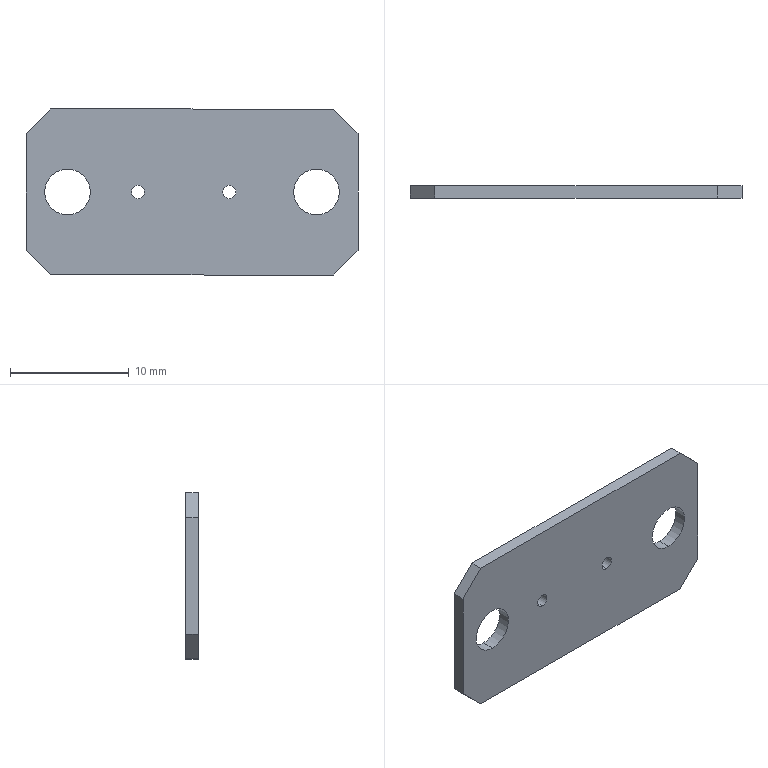Part | SolidWorks | features SplitBody 1 | 1 solid | 18 faces | box 28 x 1.05 x 14 mm | volume 375.823 mm3 | plane 10 | cylinder 8 | commonest cylinder face diameters 1.12 x4 3.85 x4
STEP:
#1=CARTESIAN_POINT('',(336.575,257.909,-266.241));
#2=VERTEX_POINT('',#1);
#3=CARTESIAN_POINT('',(336.575,257.909,-262.391));
#4=VERTEX_POINT('',#3);
#5=CARTESIAN_POINT('',(336.575,257.909,-264.316));
#6=DIRECTION('',(0.,-1.,0.));
#7=DIRECTION('',(0.,0.,1.));
#8=AXIS2_PLACEMENT_3D('',#5,#6,#7);
#9=CIRCLE('',#8,1.925);
#10=EDGE_CURVE('',#2,#4,#9,.T.);
#11=ORIENTED_EDGE('',*,*,#10,.F.);
#12=CARTESIAN_POINT('',(336.575,256.859,-266.241));
#13=VERTEX_POINT('',#12);
#14=CARTESIAN_POINT('',(336.575,263.859,-266.241));
#15=DIRECTION('',(0.,-1.,0.));
#16=VECTOR('',#15,1000.);
#17=LINE('',#14,#16);
#18=EDGE_CURVE('',#2,#13,#17,.T.);
#19=ORIENTED_EDGE('',*,*,#18,.T.);
#20=CARTESIAN_POINT('',(336.575,256.859,-262.391));
#21=VERTEX_POINT('',#20);
#22=CARTESIAN_POINT('',(336.575,256.859,-264.316));
#23=DIRECTION('',(0.,-1.,0.));
#24=DIRECTION('',(0.,0.,1.));
#25=AXIS2_PLACEMENT_3D('',#22,#23,#24);
#26=CIRCLE('',#25,1.925);
#27=EDGE_CURVE('',#13,#21,#26,.T.);
#28=ORIENTED_EDGE('',*,*,#27,.T.);
#29=CARTESIAN_POINT('',(336.575,263.859,-262.391));
#30=DIRECTION('',(0.,-1.,0.));
#31=VECTOR('',#30,1000.);
#32=LINE('',#29,#31);
#33=EDGE_CURVE('',#4,#21,#32,.T.);
#34=ORIENTED_EDGE('',*,*,#33,.F.);
#35=EDGE_LOOP('',(#11,#19,#28,#34));
#36=FACE_OUTER_BOUND('',#35,.T.);
#37=CARTESIAN_POINT('',(336.575,263.859,-264.316));
#38=DIRECTION('',(0.,-1.,0.));
#39=DIRECTION('',(0.,0.,1.));
#40=AXIS2_PLACEMENT_3D('',#37,#38,#39);
#41=CYLINDRICAL_SURFACE('',#40,1.925);
#42=ADVANCED_FACE('',(#36),#41,.F.);
#43=CARTESIAN_POINT('',(315.575,257.909,-266.241));
#44=VERTEX_POINT('',#43);
#45=CARTESIAN_POINT('',(315.575,257.909,-262.391));
#46=VERTEX_POINT('',#45);
#47=CARTESIAN_POINT('',(315.575,257.909,-264.316));
#48=DIRECTION('',(0.,-1.,0.));
#49=DIRECTION('',(0.,0.,1.));
#50=AXIS2_PLACEMENT_3D('',#47,#48,#49);
#51=CIRCLE('',#50,1.925);
#52=EDGE_CURVE('',#44,#46,#51,.T.);
#53=ORIENTED_EDGE('',*,*,#52,.F.);
#54=CARTESIAN_POINT('',(315.575,256.859,-266.241));
#55=VERTEX_POINT('',#54);
#56=CARTESIAN_POINT('',(315.575,263.859,-266.241));
#57=DIRECTION('',(0.,-1.,0.));
#58=VECTOR('',#57,1000.);
#59=LINE('',#56,#58);
#60=EDGE_CURVE('',#44,#55,#59,.T.);
#61=ORIENTED_EDGE('',*,*,#60,.T.);
#62=CARTESIAN_POINT('',(315.575,256.859,-262.391));
#63=VERTEX_POINT('',#62);
#64=CARTESIAN_POINT('',(315.575,256.859,-264.316));
#65=DIRECTION('',(0.,-1.,0.));
#66=DIRECTION('',(0.,0.,1.));
#67=AXIS2_PLACEMENT_3D('',#64,#65,#66);
#68=CIRCLE('',#67,1.925);
#69=EDGE_CURVE('',#55,#63,#68,.T.);
#70=ORIENTED_EDGE('',*,*,#69,.T.);
#71=CARTESIAN_POINT('',(315.575,263.859,-262.391));
#72=DIRECTION('',(0.,-1.,0.));
#73=VECTOR('',#72,1000.);
#74=LINE('',#71,#73);
#75=EDGE_CURVE('',#46,#63,#74,.T.);
#76=ORIENTED_EDGE('',*,*,#75,.F.);
#77=EDGE_LOOP('',(#53,#61,#70,#76));
#78=FACE_OUTER_BOUND('',#77,.T.);
#79=CARTESIAN_POINT('',(315.575,263.859,-264.316));
#80=DIRECTION('',(0.,-1.,0.));
#81=DIRECTION('',(0.,0.,1.));
#82=AXIS2_PLACEMENT_3D('',#79,#80,#81);
#83=CYLINDRICAL_SURFACE('',#82,1.925);
#84=ADVANCED_FACE('',(#78),#83,.F.);
#85=CARTESIAN_POINT('',(321.525,257.909,-264.876));
#86=VERTEX_POINT('',#85);
#87=CARTESIAN_POINT('',(321.525,257.909,-263.756));
#88=VERTEX_POINT('',#87);
#89=CARTESIAN_POINT('',(321.525,257.909,-264.316));
#90=DIRECTION('',(0.,-1.,0.));
#91=DIRECTION('',(0.,0.,1.));
#92=AXIS2_PLACEMENT_3D('',#89,#90,#91);
#93=CIRCLE('',#92,0.56);
#94=EDGE_CURVE('',#86,#88,#93,.T.);
#95=ORIENTED_EDGE('',*,*,#94,.F.);
#96=CARTESIAN_POINT('',(321.525,256.859,-264.876));
#97=VERTEX_POINT('',#96);
#98=CARTESIAN_POINT('',(321.525,256.859,-264.876));
#99=DIRECTION('',(0.,-1.,0.));
#100=VECTOR('',#99,1000.);
#101=LINE('',#98,#100);
#102=EDGE_CURVE('',#86,#97,#101,.T.);
#103=ORIENTED_EDGE('',*,*,#102,.T.);
#104=CARTESIAN_POINT('',(321.525,256.859,-263.756));
#105=VERTEX_POINT('',#104);
#106=CARTESIAN_POINT('',(321.525,256.859,-264.316));
#107=DIRECTION('',(0.,-1.,0.));
#108=DIRECTION('',(0.,0.,1.));
#109=AXIS2_PLACEMENT_3D('',#106,#107,#108);
#110=CIRCLE('',#109,0.56);
#111=EDGE_CURVE('',#97,#105,#110,.T.);
#112=ORIENTED_EDGE('',*,*,#111,.T.);
#113=CARTESIAN_POINT('',(321.525,256.859,-263.756));
#114=DIRECTION('',(0.,-1.,0.));
#115=VECTOR('',#114,1000.);
#116=LINE('',#113,#115);
#117=EDGE_CURVE('',#88,#105,#116,.T.);
#118=ORIENTED_EDGE('',*,*,#117,.F.);
#119=EDGE_LOOP('',(#95,#103,#112,#118));
#120=FACE_OUTER_BOUND('',#119,.T.);
#121=CARTESIAN_POINT('',(321.525,256.859,-264.316));
#122=DIRECTION('',(0.,-1.,0.));
#123=DIRECTION('',(0.,0.,1.));
#124=AXIS2_PLACEMENT_3D('',#121,#122,#123);
#125=CYLINDRICAL_SURFACE('',#124,0.56);
#126=ADVANCED_FACE('',(#120),#125,.F.);
#127=CARTESIAN_POINT('',(329.225,257.909,-264.876));
#128=VERTEX_POINT('',#127);
#129=CARTESIAN_POINT('',(329.225,257.909,-263.756));
#130=VERTEX_POINT('',#129);
#131=CARTESIAN_POINT('',(329.225,257.909,-264.316));
#132=DIRECTION('',(0.,-1.,0.));
#133=DIRECTION('',(0.,0.,1.));
#134=AXIS2_PLACEMENT_3D('',#131,#132,#133);
#135=CIRCLE('',#134,0.56);
#136=EDGE_CURVE('',#128,#130,#135,.T.);
#137=ORIENTED_EDGE('',*,*,#136,.F.);
#138=CARTESIAN_POINT('',(329.225,256.859,-264.876));
#139=VERTEX_POINT('',#138);
#140=CARTESIAN_POINT('',(329.225,256.859,-264.876));
#141=DIRECTION('',(0.,-1.,0.));
#142=VECTOR('',#141,1000.);
#143=LINE('',#140,#142);
#144=EDGE_CURVE('',#128,#139,#143,.T.);
#145=ORIENTED_EDGE('',*,*,#144,.T.);
#146=CARTESIAN_POINT('',(329.225,256.859,-263.756));
#147=VERTEX_POINT('',#146);
#148=CARTESIAN_POINT('',(329.225,256.859,-264.316));
#149=DIRECTION('',(0.,-1.,0.));
#150=DIRECTION('',(0.,0.,1.));
#151=AXIS2_PLACEMENT_3D('',#148,#149,#150);
#152=CIRCLE('',#151,0.56);
#153=EDGE_CURVE('',#139,#147,#152,.T.);
#154=ORIENTED_EDGE('',*,*,#153,.T.);
#155=CARTESIAN_POINT('',(329.225,256.859,-263.756));
#156=DIRECTION('',(0.,-1.,0.));
#157=VECTOR('',#156,1000.);
#158=LINE('',#155,#157);
#159=EDGE_CURVE('',#130,#147,#158,.T.);
#160=ORIENTED_EDGE('',*,*,#159,.F.);
#161=EDGE_LOOP('',(#137,#145,#154,#160));
#162=FACE_OUTER_BOUND('',#161,.T.);
#163=CARTESIAN_POINT('',(329.225,256.859,-264.316));
#164=DIRECTION('',(0.,-1.,0.));
#165=DIRECTION('',(0.,0.,1.));
#166=AXIS2_PLACEMENT_3D('',#163,#164,#165);
#167=CYLINDRICAL_SURFACE('',#166,0.56);
#168=ADVANCED_FACE('',(#162),#167,.F.);
#169=CARTESIAN_POINT('',(314.175,256.859,-271.316));
#170=VERTEX_POINT('',#169);
#171=CARTESIAN_POINT('',(337.975,256.859,-271.316));
#172=VERTEX_POINT('',#171);
#173=CARTESIAN_POINT('',(312.075,256.859,-271.316));
#174=DIRECTION('',(1.,0.,0.));
#175=VECTOR('',#174,1000.);
#176=LINE('',#173,#175);
#177=EDGE_CURVE('',#170,#172,#176,.T.);
#178=ORIENTED_EDGE('',*,*,#177,.F.);
#179=CARTESIAN_POINT('',(314.175,257.909,-271.316));
#180=VERTEX_POINT('',#179);
#181=CARTESIAN_POINT('',(314.175,256.859,-271.316));
#182=DIRECTION('',(0.,1.,0.));
#183=VECTOR('',#182,1000.);
#184=LINE('',#181,#183);
#185=EDGE_CURVE('',#170,#180,#184,.T.);
#186=ORIENTED_EDGE('',*,*,#185,.T.);
#187=CARTESIAN_POINT('',(337.975,257.909,-271.316));
#188=VERTEX_POINT('',#187);
#189=CARTESIAN_POINT('',(312.075,257.909,-271.316));
#190=DIRECTION('',(1.,0.,0.));
#191=VECTOR('',#190,1000.);
#192=LINE('',#189,#191);
#193=EDGE_CURVE('',#180,#188,#192,.T.);
#194=ORIENTED_EDGE('',*,*,#193,.T.);
#195=CARTESIAN_POINT('',(337.975,256.859,-271.316));
#196=DIRECTION('',(0.,-1.,0.));
#197=VECTOR('',#196,1000.);
#198=LINE('',#195,#197);
#199=EDGE_CURVE('',#188,#172,#198,.T.);
#200=ORIENTED_EDGE('',*,*,#199,.T.);
#201=EDGE_LOOP('',(#178,#186,#194,#200));
#202=FACE_OUTER_BOUND('',#201,.T.);
#203=CARTESIAN_POINT('',(312.075,256.859,-271.316));
#204=DIRECTION('',(0.,0.,1.));
#205=DIRECTION('',(-1.,0.,0.));
#206=AXIS2_PLACEMENT_3D('',#203,#204,#205);
#207=PLANE('',#206);
#208=ADVANCED_FACE('',(#202),#207,.F.);
#209=CARTESIAN_POINT('',(340.075,257.909,-269.216));
#210=VERTEX_POINT('',#209);
#211=CARTESIAN_POINT('',(340.075,257.909,-259.416));
#212=VERTEX_POINT('',#211);
#213=CARTESIAN_POINT('',(340.075,257.909,-271.316));
#214=DIRECTION('',(0.,0.,1.));
#215=VECTOR('',#214,1000.);
#216=LINE('',#213,#215);
#217=EDGE_CURVE('',#210,#212,#216,.T.);
#218=ORIENTED_EDGE('',*,*,#217,.T.);
#219=CARTESIAN_POINT('',(340.075,256.859,-259.416));
#220=VERTEX_POINT('',#219);
#221=CARTESIAN_POINT('',(340.075,256.859,-259.416));
#222=DIRECTION('',(0.,-1.,0.));
#223=VECTOR('',#222,1000.);
#224=LINE('',#221,#223);
#225=EDGE_CURVE('',#212,#220,#224,.T.);
#226=ORIENTED_EDGE('',*,*,#225,.T.);
#227=CARTESIAN_POINT('',(340.075,256.859,-269.216));
#228=VERTEX_POINT('',#227);
#229=CARTESIAN_POINT('',(340.075,256.859,-271.316));
#230=DIRECTION('',(0.,0.,1.));
#231=VECTOR('',#230,1000.);
#232=LINE('',#229,#231);
#233=EDGE_CURVE('',#228,#220,#232,.T.);
#234=ORIENTED_EDGE('',*,*,#233,.F.);
#235=CARTESIAN_POINT('',(340.075,256.859,-269.216));
#236=DIRECTION('',(0.,1.,0.));
#237=VECTOR('',#236,1000.);
#238=LINE('',#235,#237);
#239=EDGE_CURVE('',#228,#210,#238,.T.);
#240=ORIENTED_EDGE('',*,*,#239,.T.);
#241=EDGE_LOOP('',(#218,#226,#234,#240));
#242=FACE_OUTER_BOUND('',#241,.T.);
#243=CARTESIAN_POINT('',(340.075,256.859,-271.316));
#244=DIRECTION('',(-1.,0.,0.));
#245=DIRECTION('',(0.,-1.,0.));
#246=AXIS2_PLACEMENT_3D('',#243,#244,#245);
#247=PLANE('',#246);
#248=ADVANCED_FACE('',(#242),#247,.F.);
#249=CARTESIAN_POINT('',(337.975,257.909,-257.316));
#250=VERTEX_POINT('',#249);
#251=CARTESIAN_POINT('',(314.175,257.909,-257.316));
#252=VERTEX_POINT('',#251);
#253=CARTESIAN_POINT('',(312.075,257.909,-257.316));
#254=DIRECTION('',(-1.,0.,0.));
#255=VECTOR('',#254,1000.);
#256=LINE('',#253,#255);
#257=EDGE_CURVE('',#250,#252,#256,.T.);
#258=ORIENTED_EDGE('',*,*,#257,.T.);
#259=CARTESIAN_POINT('',(314.175,256.859,-257.316));
#260=VERTEX_POINT('',#259);
#261=CARTESIAN_POINT('',(314.175,256.859,-257.316));
#262=DIRECTION('',(0.,-1.,0.));
#263=VECTOR('',#262,1000.);
#264=LINE('',#261,#263);
#265=EDGE_CURVE('',#252,#260,#264,.T.);
#266=ORIENTED_EDGE('',*,*,#265,.T.);
#267=CARTESIAN_POINT('',(337.975,256.859,-257.316));
#268=VERTEX_POINT('',#267);
#269=CARTESIAN_POINT('',(312.075,256.859,-257.316));
#270=DIRECTION('',(-1.,0.,0.));
#271=VECTOR('',#270,1000.);
#272=LINE('',#269,#271);
#273=EDGE_CURVE('',#268,#260,#272,.T.);
#274=ORIENTED_EDGE('',*,*,#273,.F.);
#275=CARTESIAN_POINT('',(337.975,256.859,-257.316));
#276=DIRECTION('',(0.,1.,0.));
#277=VECTOR('',#276,1000.);
#278=LINE('',#275,#277);
#279=EDGE_CURVE('',#268,#250,#278,.T.);
#280=ORIENTED_EDGE('',*,*,#279,.T.);
#281=EDGE_LOOP('',(#258,#266,#274,#280));
#282=FACE_OUTER_BOUND('',#281,.T.);
#283=CARTESIAN_POINT('',(312.075,256.859,-257.316));
#284=DIRECTION('',(0.,0.,-1.));
#285=DIRECTION('',(1.,0.,0.));
#286=AXIS2_PLACEMENT_3D('',#283,#284,#285);
#287=PLANE('',#286);
#288=ADVANCED_FACE('',(#282),#287,.F.);
#289=CARTESIAN_POINT('',(312.075,257.909,-259.416));
#290=VERTEX_POINT('',#289);
#291=CARTESIAN_POINT('',(312.075,257.909,-269.216));
#292=VERTEX_POINT('',#291);
#293=CARTESIAN_POINT('',(312.075,257.909,-271.316));
#294=DIRECTION('',(0.,0.,-1.));
#295=VECTOR('',#294,1000.);
#296=LINE('',#293,#295);
#297=EDGE_CURVE('',#290,#292,#296,.T.);
#298=ORIENTED_EDGE('',*,*,#297,.T.);
#299=CARTESIAN_POINT('',(312.075,256.859,-269.216));
#300=VERTEX_POINT('',#299);
#301=CARTESIAN_POINT('',(312.075,256.859,-269.216));
#302=DIRECTION('',(0.,-1.,0.));
#303=VECTOR('',#302,1000.);
#304=LINE('',#301,#303);
#305=EDGE_CURVE('',#292,#300,#304,.T.);
#306=ORIENTED_EDGE('',*,*,#305,.T.);
#307=CARTESIAN_POINT('',(312.075,256.859,-259.416));
#308=VERTEX_POINT('',#307);
#309=CARTESIAN_POINT('',(312.075,256.859,-271.316));
#310=DIRECTION('',(0.,0.,-1.));
#311=VECTOR('',#310,1000.);
#312=LINE('',#309,#311);
#313=EDGE_CURVE('',#308,#300,#312,.T.);
#314=ORIENTED_EDGE('',*,*,#313,.F.);
#315=CARTESIAN_POINT('',(312.075,256.859,-259.416));
#316=DIRECTION('',(0.,1.,0.));
#317=VECTOR('',#316,1000.);
#318=LINE('',#315,#317);
#319=EDGE_CURVE('',#308,#290,#318,.T.);
#320=ORIENTED_EDGE('',*,*,#319,.T.);
#321=EDGE_LOOP('',(#298,#306,#314,#320));
#322=FACE_OUTER_BOUND('',#321,.T.);
#323=CARTESIAN_POINT('',(312.075,256.859,-271.316));
#324=DIRECTION('',(1.,0.,0.));
#325=DIRECTION('',(0.,1.,0.));
#326=AXIS2_PLACEMENT_3D('',#323,#324,#325);
#327=PLANE('',#326);
#328=ADVANCED_FACE('',(#322),#327,.F.);
#329=CARTESIAN_POINT('',(336.575,256.859,-264.316));
#330=DIRECTION('',(0.,-1.,0.));
#331=DIRECTION('',(0.,0.,1.));
#332=AXIS2_PLACEMENT_3D('',#329,#330,#331);
#333=CIRCLE('',#332,1.925);
#334=EDGE_CURVE('',#21,#13,#333,.T.);
#335=ORIENTED_EDGE('',*,*,#334,.F.);
#336=ORIENTED_EDGE('',*,*,#27,.F.);
#337=EDGE_LOOP('',(#335,#336));
#338=FACE_BOUND('',#337,.T.);
#339=CARTESIAN_POINT('',(315.575,256.859,-264.316));
#340=DIRECTION('',(0.,-1.,0.));
#341=DIRECTION('',(0.,0.,1.));
#342=AXIS2_PLACEMENT_3D('',#339,#340,#341);
#343=CIRCLE('',#342,1.925);
#344=EDGE_CURVE('',#63,#55,#343,.T.);
#345=ORIENTED_EDGE('',*,*,#344,.F.);
#346=ORIENTED_EDGE('',*,*,#69,.F.);
#347=EDGE_LOOP('',(#345,#346));
#348=FACE_BOUND('',#347,.T.);
#349=CARTESIAN_POINT('',(321.525,256.859,-264.316));
#350=DIRECTION('',(0.,-1.,0.));
#351=DIRECTION('',(0.,0.,1.));
#352=AXIS2_PLACEMENT_3D('',#349,#350,#351);
#353=CIRCLE('',#352,0.56);
#354=EDGE_CURVE('',#105,#97,#353,.T.);
#355=ORIENTED_EDGE('',*,*,#354,.F.);
#356=ORIENTED_EDGE('',*,*,#111,.F.);
#357=EDGE_LOOP('',(#355,#356));
#358=FACE_BOUND('',#357,.T.);
#359=CARTESIAN_POINT('',(329.225,256.859,-264.316));
#360=DIRECTION('',(0.,-1.,0.));
#361=DIRECTION('',(0.,0.,1.));
#362=AXIS2_PLACEMENT_3D('',#359,#360,#361);
#363=CIRCLE('',#362,0.56);
#364=EDGE_CURVE('',#147,#139,#363,.T.);
#365=ORIENTED_EDGE('',*,*,#364,.F.);
#366=ORIENTED_EDGE('',*,*,#153,.F.);
#367=EDGE_LOOP('',(#365,#366));
#368=FACE_BOUND('',#367,.T.);
#369=ORIENTED_EDGE('',*,*,#313,.T.);
#370=CARTESIAN_POINT('',(327.125,256.859,-284.266));
#371=DIRECTION('',(0.7071,0.,-0.7071));
#372=VECTOR('',#371,1000.);
#373=LINE('',#370,#372);
#374=EDGE_CURVE('',#300,#170,#373,.T.);
#375=ORIENTED_EDGE('',*,*,#374,.T.);
#376=ORIENTED_EDGE('',*,*,#177,.T.);
#377=CARTESIAN_POINT('',(339.025,256.859,-270.266));
#378=DIRECTION('',(0.7071,0.,0.7071));
#379=VECTOR('',#378,1000.);
#380=LINE('',#377,#379);
#381=EDGE_CURVE('',#172,#228,#380,.T.);
#382=ORIENTED_EDGE('',*,*,#381,.T.);
#383=ORIENTED_EDGE('',*,*,#233,.T.);
#384=CARTESIAN_POINT('',(346.025,256.859,-265.366));
#385=DIRECTION('',(-0.7071,0.,0.7071));
#386=VECTOR('',#385,1000.);
#387=LINE('',#384,#386);
#388=EDGE_CURVE('',#220,#268,#387,.T.);
#389=ORIENTED_EDGE('',*,*,#388,.T.);
#390=ORIENTED_EDGE('',*,*,#273,.T.);
#391=CARTESIAN_POINT('',(320.125,256.859,-251.366));
#392=DIRECTION('',(-0.7071,0.,-0.7071));
#393=VECTOR('',#392,1000.);
#394=LINE('',#391,#393);
#395=EDGE_CURVE('',#260,#308,#394,.T.);
#396=ORIENTED_EDGE('',*,*,#395,.T.);
#397=EDGE_LOOP('',(#369,#375,#376,#382,#383,#389,#390,#396));
#398=FACE_OUTER_BOUND('',#397,.T.);
#399=CARTESIAN_POINT('',(340.075,256.859,-271.316));
#400=DIRECTION('',(0.,-1.,0.));
#401=DIRECTION('',(0.,0.,1.));
#402=AXIS2_PLACEMENT_3D('',#399,#400,#401);
#403=PLANE('',#402);
#404=ADVANCED_FACE('',(#338,#348,#358,#368,#398),#403,.T.);
#405=CARTESIAN_POINT('',(336.575,257.909,-264.316));
#406=DIRECTION('',(0.,-1.,0.));
#407=DIRECTION('',(0.,0.,1.));
#408=AXIS2_PLACEMENT_3D('',#405,#406,#407);
#409=CIRCLE('',#408,1.925);
#410=EDGE_CURVE('',#4,#2,#409,.T.);
#411=ORIENTED_EDGE('',*,*,#410,.T.);
#412=ORIENTED_EDGE('',*,*,#10,.T.);
#413=EDGE_LOOP('',(#411,#412));
#414=FACE_BOUND('',#413,.T.);
#415=CARTESIAN_POINT('',(315.575,257.909,-264.316));
#416=DIRECTION('',(0.,-1.,0.));
#417=DIRECTION('',(0.,0.,1.));
#418=AXIS2_PLACEMENT_3D('',#415,#416,#417);
#419=CIRCLE('',#418,1.925);
#420=EDGE_CURVE('',#46,#44,#419,.T.);
#421=ORIENTED_EDGE('',*,*,#420,.T.);
#422=ORIENTED_EDGE('',*,*,#52,.T.);
#423=EDGE_LOOP('',(#421,#422));
#424=FACE_BOUND('',#423,.T.);
#425=CARTESIAN_POINT('',(321.525,257.909,-264.316));
#426=DIRECTION('',(0.,-1.,0.));
#427=DIRECTION('',(0.,0.,1.));
#428=AXIS2_PLACEMENT_3D('',#425,#426,#427);
#429=CIRCLE('',#428,0.56);
#430=EDGE_CURVE('',#88,#86,#429,.T.);
#431=ORIENTED_EDGE('',*,*,#430,.T.);
#432=ORIENTED_EDGE('',*,*,#94,.T.);
#433=EDGE_LOOP('',(#431,#432));
#434=FACE_BOUND('',#433,.T.);
#435=CARTESIAN_POINT('',(329.225,257.909,-264.316));
#436=DIRECTION('',(0.,-1.,0.));
#437=DIRECTION('',(0.,0.,1.));
#438=AXIS2_PLACEMENT_3D('',#435,#436,#437);
#439=CIRCLE('',#438,0.56);
#440=EDGE_CURVE('',#130,#128,#439,.T.);
#441=ORIENTED_EDGE('',*,*,#440,.T.);
#442=ORIENTED_EDGE('',*,*,#136,.T.);
#443=EDGE_LOOP('',(#441,#442));
#444=FACE_BOUND('',#443,.T.);
#445=ORIENTED_EDGE('',*,*,#193,.F.);
#446=CARTESIAN_POINT('',(314.175,257.909,-271.316));
#447=DIRECTION('',(-0.7071,0.,0.7071));
#448=VECTOR('',#447,1000.);
#449=LINE('',#446,#448);
#450=EDGE_CURVE('',#180,#292,#449,.T.);
#451=ORIENTED_EDGE('',*,*,#450,.T.);
#452=ORIENTED_EDGE('',*,*,#297,.F.);
#453=CARTESIAN_POINT('',(312.075,257.909,-259.416));
#454=DIRECTION('',(0.7071,0.,0.7071));
#455=VECTOR('',#454,1000.);
#456=LINE('',#453,#455);
#457=EDGE_CURVE('',#290,#252,#456,.T.);
#458=ORIENTED_EDGE('',*,*,#457,.T.);
#459=ORIENTED_EDGE('',*,*,#257,.F.);
#460=CARTESIAN_POINT('',(337.975,257.909,-257.316));
#461=DIRECTION('',(0.7071,0.,-0.7071));
#462=VECTOR('',#461,1000.);
#463=LINE('',#460,#462);
#464=EDGE_CURVE('',#250,#212,#463,.T.);
#465=ORIENTED_EDGE('',*,*,#464,.T.);
#466=ORIENTED_EDGE('',*,*,#217,.F.);
#467=CARTESIAN_POINT('',(340.075,257.909,-269.216));
#468=DIRECTION('',(-0.7071,0.,-0.7071));
#469=VECTOR('',#468,1000.);
#470=LINE('',#467,#469);
#471=EDGE_CURVE('',#210,#188,#470,.T.);
#472=ORIENTED_EDGE('',*,*,#471,.T.);
#473=EDGE_LOOP('',(#445,#451,#452,#458,#459,#465,#466,#472));
#474=FACE_OUTER_BOUND('',#473,.T.);
#475=CARTESIAN_POINT('',(340.075,257.909,-271.316));
#476=DIRECTION('',(0.,-1.,0.));
#477=DIRECTION('',(0.,0.,1.));
#478=AXIS2_PLACEMENT_3D('',#475,#476,#477);
#479=PLANE('',#478);
#480=ADVANCED_FACE('',(#414,#424,#434,#444,#474),#479,.F.);
#481=ORIENTED_EDGE('',*,*,#144,.F.);
#482=ORIENTED_EDGE('',*,*,#440,.F.);
#483=ORIENTED_EDGE('',*,*,#159,.T.);
#484=ORIENTED_EDGE('',*,*,#364,.T.);
#485=EDGE_LOOP('',(#481,#482,#483,#484));
#486=FACE_OUTER_BOUND('',#485,.T.);
#487=CARTESIAN_POINT('',(329.225,256.859,-264.316));
#488=DIRECTION('',(0.,-1.,0.));
#489=DIRECTION('',(0.,0.,1.));
#490=AXIS2_PLACEMENT_3D('',#487,#488,#489);
#491=CYLINDRICAL_SURFACE('',#490,0.56);
#492=ADVANCED_FACE('',(#486),#491,.F.);
#493=ORIENTED_EDGE('',*,*,#102,.F.);
#494=ORIENTED_EDGE('',*,*,#430,.F.);
#495=ORIENTED_EDGE('',*,*,#117,.T.);
#496=ORIENTED_EDGE('',*,*,#354,.T.);
#497=EDGE_LOOP('',(#493,#494,#495,#496));
#498=FACE_OUTER_BOUND('',#497,.T.);
#499=CARTESIAN_POINT('',(321.525,256.859,-264.316));
#500=DIRECTION('',(0.,-1.,0.));
#501=DIRECTION('',(0.,0.,1.));
#502=AXIS2_PLACEMENT_3D('',#499,#500,#501);
#503=CYLINDRICAL_SURFACE('',#502,0.56);
#504=ADVANCED_FACE('',(#498),#503,.F.);
#505=ORIENTED_EDGE('',*,*,#60,.F.);
#506=ORIENTED_EDGE('',*,*,#420,.F.);
#507=ORIENTED_EDGE('',*,*,#75,.T.);
#508=ORIENTED_EDGE('',*,*,#344,.T.);
#509=EDGE_LOOP('',(#505,#506,#507,#508));
#510=FACE_OUTER_BOUND('',#509,.T.);
#511=CARTESIAN_POINT('',(315.575,263.859,-264.316));
#512=DIRECTION('',(0.,-1.,0.));
#513=DIRECTION('',(0.,0.,1.));
#514=AXIS2_PLACEMENT_3D('',#511,#512,#513);
#515=CYLINDRICAL_SURFACE('',#514,1.925);
#516=ADVANCED_FACE('',(#510),#515,.F.);
#517=ORIENTED_EDGE('',*,*,#18,.F.);
#518=ORIENTED_EDGE('',*,*,#410,.F.);
#519=ORIENTED_EDGE('',*,*,#33,.T.);
#520=ORIENTED_EDGE('',*,*,#334,.T.);
#521=EDGE_LOOP('',(#517,#518,#519,#520));
#522=FACE_OUTER_BOUND('',#521,.T.);
#523=CARTESIAN_POINT('',(336.575,263.859,-264.316));
#524=DIRECTION('',(0.,-1.,0.));
#525=DIRECTION('',(0.,0.,1.));
#526=AXIS2_PLACEMENT_3D('',#523,#524,#525);
#527=CYLINDRICAL_SURFACE('',#526,1.925);
#528=ADVANCED_FACE('',(#522),#527,.F.);
#529=ORIENTED_EDGE('',*,*,#374,.F.);
#530=ORIENTED_EDGE('',*,*,#305,.F.);
#531=ORIENTED_EDGE('',*,*,#450,.F.);
#532=ORIENTED_EDGE('',*,*,#185,.F.);
#533=EDGE_LOOP('',(#529,#530,#531,#532));
#534=FACE_OUTER_BOUND('',#533,.T.);
#535=CARTESIAN_POINT('',(314.175,256.859,-271.316));
#536=DIRECTION('',(0.7071,0.,0.7071));
#537=DIRECTION('',(-0.7071,0.,0.7071));
#538=AXIS2_PLACEMENT_3D('',#535,#536,#537);
#539=PLANE('',#538);
#540=ADVANCED_FACE('',(#534),#539,.F.);
#541=ORIENTED_EDGE('',*,*,#395,.F.);
#542=ORIENTED_EDGE('',*,*,#265,.F.);
#543=ORIENTED_EDGE('',*,*,#457,.F.);
#544=ORIENTED_EDGE('',*,*,#319,.F.);
#545=EDGE_LOOP('',(#541,#542,#543,#544));
#546=FACE_OUTER_BOUND('',#545,.T.);
#547=CARTESIAN_POINT('',(312.075,256.859,-259.416));
#548=DIRECTION('',(0.7071,0.,-0.7071));
#549=DIRECTION('',(0.7071,0.,0.7071));
#550=AXIS2_PLACEMENT_3D('',#547,#548,#549);
#551=PLANE('',#550);
#552=ADVANCED_FACE('',(#546),#551,.F.);
#553=ORIENTED_EDGE('',*,*,#388,.F.);
#554=ORIENTED_EDGE('',*,*,#225,.F.);
#555=ORIENTED_EDGE('',*,*,#464,.F.);
#556=ORIENTED_EDGE('',*,*,#279,.F.);
#557=EDGE_LOOP('',(#553,#554,#555,#556));
#558=FACE_OUTER_BOUND('',#557,.T.);
#559=CARTESIAN_POINT('',(337.975,256.859,-257.316));
#560=DIRECTION('',(-0.7071,0.,-0.7071));
#561=DIRECTION('',(0.7071,0.,-0.7071));
#562=AXIS2_PLACEMENT_3D('',#559,#560,#561);
#563=PLANE('',#562);
#564=ADVANCED_FACE('',(#558),#563,.F.);
#565=ORIENTED_EDGE('',*,*,#381,.F.);
#566=ORIENTED_EDGE('',*,*,#199,.F.);
#567=ORIENTED_EDGE('',*,*,#471,.F.);
#568=ORIENTED_EDGE('',*,*,#239,.F.);
#569=EDGE_LOOP('',(#565,#566,#567,#568));
#570=FACE_OUTER_BOUND('',#569,.T.);
#571=CARTESIAN_POINT('',(340.075,256.859,-269.216));
#572=DIRECTION('',(-0.7071,0.,0.7071));
#573=DIRECTION('',(-0.7071,0.,-0.7071));
#574=AXIS2_PLACEMENT_3D('',#571,#572,#573);
#575=PLANE('',#574);
#576=ADVANCED_FACE('',(#570),#575,.F.);
#577=CLOSED_SHELL('',(#42,#84,#126,#168,#208,#248,#288,#328,#404,#480,#492,#504,#516,#528,#540,#552,#564,#576));
#578=MANIFOLD_SOLID_BREP('',#577);
#579=CARTESIAN_POINT('',(0.,0.,0.));
#580=DIRECTION('',(0.,0.,1.));
#581=DIRECTION('',(1.,0.,0.));
#582=AXIS2_PLACEMENT_3D('',#579,#580,#581);
#583=(LENGTH_UNIT()NAMED_UNIT(*)SI_UNIT(.MILLI.,.METRE.));
#584=UNCERTAINTY_MEASURE_WITH_UNIT(LENGTH_MEASURE(0.00001),#583,'','');
#585=(NAMED_UNIT(*)PLANE_ANGLE_UNIT()SI_UNIT($,.RADIAN.));
#586=(NAMED_UNIT(*)SI_UNIT($,.STERADIAN.)SOLID_ANGLE_UNIT());
#587=(GEOMETRIC_REPRESENTATION_CONTEXT(3)GLOBAL_UNCERTAINTY_ASSIGNED_CONTEXT((#584))GLOBAL_UNIT_ASSIGNED_CONTEXT((#583,#585,#586))REPRESENTATION_CONTEXT('',''));
#588=ADVANCED_BREP_SHAPE_REPRESENTATION('',(#578,#582),#587);